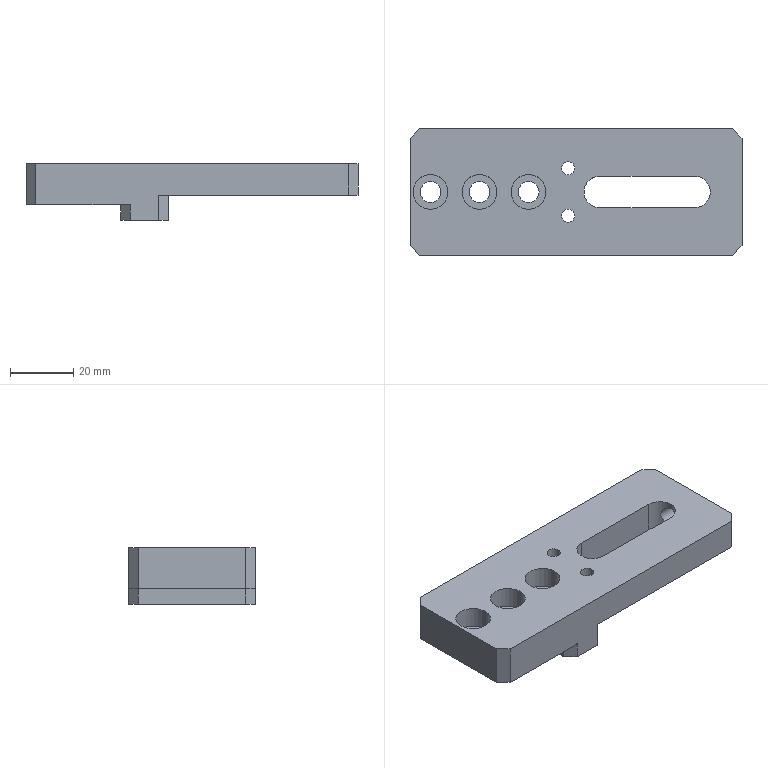Part | SolidWorks | features HoleWzd 3, ICE 3, Chamfer 1, Cut 1, Extrusion 1 | 1 solid | 47 faces | box 105 x 40 x 18 mm | volume 42827 mm3 | plane 24 | cylinder 23 | commonest cylinder face diameters 6.6 x8 11 x6 10 x5 4.2 x4
STEP:
#1=CARTESIAN_POINT('',(-0.4,7.5,8.));
#2=VERTEX_POINT('',#1);
#3=CARTESIAN_POINT('',(-4.6,7.5,8.));
#4=VERTEX_POINT('',#3);
#5=CARTESIAN_POINT('',(-2.5,7.5,8.));
#6=DIRECTION('',(0.,0.,-1.));
#7=DIRECTION('',(-1.,0.,0.));
#8=AXIS2_PLACEMENT_3D('',#5,#6,#7);
#9=CIRCLE('',#8,2.1);
#10=EDGE_CURVE('',#2,#4,#9,.T.);
#11=ORIENTED_EDGE('',*,*,#10,.T.);
#12=CARTESIAN_POINT('',(-4.6,7.5,18.));
#13=VERTEX_POINT('',#12);
#14=CARTESIAN_POINT('',(-4.6,7.5,18.));
#15=DIRECTION('',(0.,0.,1.));
#16=VECTOR('',#15,1000.);
#17=LINE('',#14,#16);
#18=EDGE_CURVE('',#4,#13,#17,.T.);
#19=ORIENTED_EDGE('',*,*,#18,.T.);
#20=CARTESIAN_POINT('',(-0.4,7.5,18.));
#21=VERTEX_POINT('',#20);
#22=CARTESIAN_POINT('',(-2.5,7.5,18.));
#23=DIRECTION('',(0.,0.,1.));
#24=DIRECTION('',(1.,0.,0.));
#25=AXIS2_PLACEMENT_3D('',#22,#23,#24);
#26=CIRCLE('',#25,2.1);
#27=EDGE_CURVE('',#13,#21,#26,.T.);
#28=ORIENTED_EDGE('',*,*,#27,.T.);
#29=CARTESIAN_POINT('',(-0.4,7.5,18.));
#30=DIRECTION('',(0.,0.,1.));
#31=VECTOR('',#30,1000.);
#32=LINE('',#29,#31);
#33=EDGE_CURVE('',#2,#21,#32,.T.);
#34=ORIENTED_EDGE('',*,*,#33,.F.);
#35=EDGE_LOOP('',(#11,#19,#28,#34));
#36=FACE_OUTER_BOUND('',#35,.T.);
#37=CARTESIAN_POINT('',(-2.5,7.5,18.));
#38=DIRECTION('',(0.,0.,1.));
#39=DIRECTION('',(1.,0.,0.));
#40=AXIS2_PLACEMENT_3D('',#37,#38,#39);
#41=CYLINDRICAL_SURFACE('',#40,2.1);
#42=ADVANCED_FACE('',(#36),#41,.F.);
#43=CARTESIAN_POINT('',(-0.4,-7.5,8.));
#44=VERTEX_POINT('',#43);
#45=CARTESIAN_POINT('',(-4.6,-7.5,8.));
#46=VERTEX_POINT('',#45);
#47=CARTESIAN_POINT('',(-2.5,-7.5,8.));
#48=DIRECTION('',(0.,0.,-1.));
#49=DIRECTION('',(-1.,0.,0.));
#50=AXIS2_PLACEMENT_3D('',#47,#48,#49);
#51=CIRCLE('',#50,2.1);
#52=EDGE_CURVE('',#44,#46,#51,.T.);
#53=ORIENTED_EDGE('',*,*,#52,.T.);
#54=CARTESIAN_POINT('',(-4.6,-7.5,18.));
#55=VERTEX_POINT('',#54);
#56=CARTESIAN_POINT('',(-4.6,-7.5,18.));
#57=DIRECTION('',(0.,0.,1.));
#58=VECTOR('',#57,1000.);
#59=LINE('',#56,#58);
#60=EDGE_CURVE('',#46,#55,#59,.T.);
#61=ORIENTED_EDGE('',*,*,#60,.T.);
#62=CARTESIAN_POINT('',(-0.4,-7.5,18.));
#63=VERTEX_POINT('',#62);
#64=CARTESIAN_POINT('',(-2.5,-7.5,18.));
#65=DIRECTION('',(0.,0.,1.));
#66=DIRECTION('',(1.,0.,0.));
#67=AXIS2_PLACEMENT_3D('',#64,#65,#66);
#68=CIRCLE('',#67,2.1);
#69=EDGE_CURVE('',#55,#63,#68,.T.);
#70=ORIENTED_EDGE('',*,*,#69,.T.);
#71=CARTESIAN_POINT('',(-0.4,-7.5,18.));
#72=DIRECTION('',(0.,0.,1.));
#73=VECTOR('',#72,1000.);
#74=LINE('',#71,#73);
#75=EDGE_CURVE('',#44,#63,#74,.T.);
#76=ORIENTED_EDGE('',*,*,#75,.F.);
#77=EDGE_LOOP('',(#53,#61,#70,#76));
#78=FACE_OUTER_BOUND('',#77,.T.);
#79=CARTESIAN_POINT('',(-2.5,-7.5,18.));
#80=DIRECTION('',(0.,0.,1.));
#81=DIRECTION('',(1.,0.,0.));
#82=AXIS2_PLACEMENT_3D('',#79,#80,#81);
#83=CYLINDRICAL_SURFACE('',#82,2.1);
#84=ADVANCED_FACE('',(#78),#83,.F.);
#85=CARTESIAN_POINT('',(42.5,0.,16.3));
#86=VERTEX_POINT('',#85);
#87=CARTESIAN_POINT('',(42.5,0.,9.7));
#88=VERTEX_POINT('',#87);
#89=CARTESIAN_POINT('',(42.5,0.,16.3));
#90=CARTESIAN_POINT('',(42.5,-0.222,16.3));
#91=CARTESIAN_POINT('',(42.485,-0.447,16.277));
#92=CARTESIAN_POINT('',(42.427,-0.8816,16.188));
#93=CARTESIAN_POINT('',(42.384,-1.09,16.122));
#94=CARTESIAN_POINT('',(42.277,-1.492,15.952));
#95=CARTESIAN_POINT('',(42.213,-1.681,15.848));
#96=CARTESIAN_POINT('',(42.073,-2.031,15.61));
#97=CARTESIAN_POINT('',(41.996,-2.195,15.473));
#98=CARTESIAN_POINT('',(41.84,-2.489,15.177));
#99=CARTESIAN_POINT('',(41.76,-2.621,15.016));
#100=CARTESIAN_POINT('',(41.607,-2.856,14.667));
#101=CARTESIAN_POINT('',(41.533,-2.958,14.479));
#102=CARTESIAN_POINT('',(41.406,-3.123,14.086));
#103=CARTESIAN_POINT('',(41.352,-3.189,13.878));
#104=CARTESIAN_POINT('',(41.276,-3.277,13.444));
#105=CARTESIAN_POINT('',(41.256,-3.3,13.223));
#106=CARTESIAN_POINT('',(41.256,-3.3,12.774));
#107=CARTESIAN_POINT('',(41.277,-3.277,12.55));
#108=CARTESIAN_POINT('',(41.352,-3.188,12.119));
#109=CARTESIAN_POINT('',(41.407,-3.122,11.909));
#110=CARTESIAN_POINT('',(41.598,-2.872,11.32));
#111=CARTESIAN_POINT('',(41.764,-2.633,10.967));
#112=CARTESIAN_POINT('',(41.997,-2.191,10.524));
#113=CARTESIAN_POINT('',(42.074,-2.028,10.388));
#114=CARTESIAN_POINT('',(42.214,-1.677,10.15));
#115=CARTESIAN_POINT('',(42.277,-1.49,10.048));
#116=CARTESIAN_POINT('',(42.383,-1.094,9.879));
#117=CARTESIAN_POINT('',(42.427,-0.8814,9.812));
#118=CARTESIAN_POINT('',(42.485,-0.4473,9.723));
#119=CARTESIAN_POINT('',(42.5,-0.2253,9.7));
#120=CARTESIAN_POINT('',(42.5,0.,9.7));
#121=B_SPLINE_CURVE_WITH_KNOTS('',3,(#89,#90,#91,#92,#93,#94,#95,#96,#97,#98,#99,#100,#101,#102,#103,#104,#105,#106,#107,#108,#109,#110,#111,#112,#113,#114,#115,#116,#117,#118,#119,#120),.UNSPECIFIED.,.F.,.F.,(4,2,2,2,2,2,2,2,2,2,2,2,2,2,2,4),(0.01066,0.01132,0.01199,0.01265,0.01332,0.01398,0.01465,0.01531,0.01598,0.01664,0.01731,0.01864,0.0193,0.01997,0.02063,0.0213),.UNSPECIFIED.);
#122=EDGE_CURVE('',#86,#88,#121,.T.);
#123=ORIENTED_EDGE('',*,*,#122,.F.);
#124=CARTESIAN_POINT('',(52.5,0.,16.3));
#125=VERTEX_POINT('',#124);
#126=CARTESIAN_POINT('',(52.5,0.,16.3));
#127=DIRECTION('',(1.,0.,0.));
#128=VECTOR('',#127,1000.);
#129=LINE('',#126,#128);
#130=EDGE_CURVE('',#86,#125,#129,.T.);
#131=ORIENTED_EDGE('',*,*,#130,.T.);
#132=CARTESIAN_POINT('',(52.5,0.,9.7));
#133=VERTEX_POINT('',#132);
#134=CARTESIAN_POINT('',(52.5,0.,13.));
#135=DIRECTION('',(1.,0.,0.));
#136=DIRECTION('',(0.,0.,-1.));
#137=AXIS2_PLACEMENT_3D('',#134,#135,#136);
#138=CIRCLE('',#137,3.3);
#139=EDGE_CURVE('',#125,#133,#138,.T.);
#140=ORIENTED_EDGE('',*,*,#139,.T.);
#141=CARTESIAN_POINT('',(52.5,0.,9.7));
#142=DIRECTION('',(1.,0.,0.));
#143=VECTOR('',#142,1000.);
#144=LINE('',#141,#143);
#145=EDGE_CURVE('',#88,#133,#144,.T.);
#146=ORIENTED_EDGE('',*,*,#145,.F.);
#147=EDGE_LOOP('',(#123,#131,#140,#146));
#148=FACE_OUTER_BOUND('',#147,.T.);
#149=CARTESIAN_POINT('',(52.5,0.,13.));
#150=DIRECTION('',(1.,0.,0.));
#151=DIRECTION('',(0.,0.,-1.));
#152=AXIS2_PLACEMENT_3D('',#149,#150,#151);
#153=CYLINDRICAL_SURFACE('',#152,3.3);
#154=ADVANCED_FACE('',(#148),#153,.F.);
#155=CARTESIAN_POINT('',(37.5,5.,8.));
#156=VERTEX_POINT('',#155);
#157=CARTESIAN_POINT('',(42.5,0.,8.));
#158=VERTEX_POINT('',#157);
#159=CARTESIAN_POINT('',(37.5,0.,8.));
#160=DIRECTION('',(0.,0.,-1.));
#161=DIRECTION('',(-1.,0.,0.));
#162=AXIS2_PLACEMENT_3D('',#159,#160,#161);
#163=CIRCLE('',#162,5.);
#164=EDGE_CURVE('',#156,#158,#163,.T.);
#165=ORIENTED_EDGE('',*,*,#164,.T.);
#166=CARTESIAN_POINT('',(42.5,0.,0.));
#167=DIRECTION('',(0.,0.,1.));
#168=VECTOR('',#167,1000.);
#169=LINE('',#166,#168);
#170=EDGE_CURVE('',#158,#88,#169,.T.);
#171=ORIENTED_EDGE('',*,*,#170,.T.);
#172=CARTESIAN_POINT('',(42.5,0.,9.7));
#173=CARTESIAN_POINT('',(42.5,0.2256,9.7));
#174=CARTESIAN_POINT('',(42.485,0.4462,9.723));
#175=CARTESIAN_POINT('',(42.427,0.8783,9.811));
#176=CARTESIAN_POINT('',(42.384,1.091,9.878));
#177=CARTESIAN_POINT('',(42.224,1.689,10.132));
#178=CARTESIAN_POINT('',(42.075,2.045,10.376));
#179=CARTESIAN_POINT('',(41.841,2.487,10.82));
#180=CARTESIAN_POINT('',(41.76,2.621,10.984));
#181=CARTESIAN_POINT('',(41.608,2.854,11.331));
#182=CARTESIAN_POINT('',(41.535,2.955,11.515));
#183=CARTESIAN_POINT('',(41.408,3.121,11.908));
#184=CARTESIAN_POINT('',(41.353,3.188,12.118));
#185=CARTESIAN_POINT('',(41.296,3.254,12.441));
#186=CARTESIAN_POINT('',(41.282,3.271,12.55));
#187=CARTESIAN_POINT('',(41.262,3.294,12.772));
#188=CARTESIAN_POINT('',(41.256,3.3,12.885));
#189=CARTESIAN_POINT('',(41.256,3.3,13.221));
#190=CARTESIAN_POINT('',(41.276,3.278,13.441));
#191=CARTESIAN_POINT('',(41.351,3.189,13.876));
#192=CARTESIAN_POINT('',(41.405,3.124,14.084));
#193=CARTESIAN_POINT('',(41.533,2.957,14.48));
#194=CARTESIAN_POINT('',(41.607,2.855,14.668));
#195=CARTESIAN_POINT('',(41.76,2.621,15.016));
#196=CARTESIAN_POINT('',(41.84,2.488,15.178));
#197=CARTESIAN_POINT('',(41.997,2.191,15.476));
#198=CARTESIAN_POINT('',(42.073,2.03,15.61));
#199=CARTESIAN_POINT('',(42.212,1.682,15.847));
#200=CARTESIAN_POINT('',(42.277,1.491,15.952));
#201=CARTESIAN_POINT('',(42.384,1.091,16.122));
#202=CARTESIAN_POINT('',(42.426,0.8826,16.188));
#203=CARTESIAN_POINT('',(42.485,0.4472,16.277));
#204=CARTESIAN_POINT('',(42.5,0.2223,16.3));
#205=CARTESIAN_POINT('',(42.5,0.,16.3));
#206=B_SPLINE_CURVE_WITH_KNOTS('',3,(#172,#173,#174,#175,#176,#177,#178,#179,#180,#181,#182,#183,#184,#185,#186,#187,#188,#189,#190,#191,#192,#193,#194,#195,#196,#197,#198,#199,#200,#201,#202,#203,#204,#205),.UNSPECIFIED.,.F.,.F.,(4,2,2,2,2,2,2,2,2,2,2,2,2,2,2,2,4),(0.,0.000666,0.001332,0.002664,0.00333,0.003996,0.004662,0.004995,0.005328,0.005994,0.00666,0.007326,0.007992,0.008658,0.009324,0.00999,0.01066),.UNSPECIFIED.);
#207=EDGE_CURVE('',#88,#86,#206,.T.);
#208=ORIENTED_EDGE('',*,*,#207,.T.);
#209=CARTESIAN_POINT('',(42.5,0.,18.));
#210=VERTEX_POINT('',#209);
#211=CARTESIAN_POINT('',(42.5,0.,0.));
#212=DIRECTION('',(0.,0.,1.));
#213=VECTOR('',#212,1000.);
#214=LINE('',#211,#213);
#215=EDGE_CURVE('',#86,#210,#214,.T.);
#216=ORIENTED_EDGE('',*,*,#215,.T.);
#217=CARTESIAN_POINT('',(37.5,5.,18.));
#218=VERTEX_POINT('',#217);
#219=CARTESIAN_POINT('',(37.5,0.,18.));
#220=DIRECTION('',(0.,0.,1.));
#221=DIRECTION('',(1.,0.,0.));
#222=AXIS2_PLACEMENT_3D('',#219,#220,#221);
#223=CIRCLE('',#222,5.);
#224=EDGE_CURVE('',#210,#218,#223,.T.);
#225=ORIENTED_EDGE('',*,*,#224,.T.);
#226=CARTESIAN_POINT('',(37.5,5.,0.));
#227=DIRECTION('',(0.,0.,1.));
#228=VECTOR('',#227,1000.);
#229=LINE('',#226,#228);
#230=EDGE_CURVE('',#156,#218,#229,.T.);
#231=ORIENTED_EDGE('',*,*,#230,.F.);
#232=EDGE_LOOP('',(#165,#171,#208,#216,#225,#231));
#233=FACE_OUTER_BOUND('',#232,.T.);
#234=CARTESIAN_POINT('',(37.5,0.,0.));
#235=DIRECTION('',(0.,0.,1.));
#236=DIRECTION('',(1.,0.,0.));
#237=AXIS2_PLACEMENT_3D('',#234,#235,#236);
#238=CYLINDRICAL_SURFACE('',#237,5.);
#239=ADVANCED_FACE('',(#233),#238,.F.);
#240=CARTESIAN_POINT('',(-10.,0.,2.));
#241=VERTEX_POINT('',#240);
#242=CARTESIAN_POINT('',(-20.,0.,2.));
#243=VERTEX_POINT('',#242);
#244=CARTESIAN_POINT('',(-15.,0.,2.));
#245=DIRECTION('',(0.,0.,-1.));
#246=DIRECTION('',(-1.,0.,0.));
#247=AXIS2_PLACEMENT_3D('',#244,#245,#246);
#248=CIRCLE('',#247,5.);
#249=EDGE_CURVE('',#241,#243,#248,.T.);
#250=ORIENTED_EDGE('',*,*,#249,.F.);
#251=CARTESIAN_POINT('',(-10.,0.,0.));
#252=VERTEX_POINT('',#251);
#253=CARTESIAN_POINT('',(-10.,0.,2.));
#254=DIRECTION('',(0.,0.,-1.));
#255=VECTOR('',#254,1000.);
#256=LINE('',#253,#255);
#257=EDGE_CURVE('',#241,#252,#256,.T.);
#258=ORIENTED_EDGE('',*,*,#257,.T.);
#259=CARTESIAN_POINT('',(-20.,0.,0.));
#260=VERTEX_POINT('',#259);
#261=CARTESIAN_POINT('',(-15.,0.,0.));
#262=DIRECTION('',(0.,0.,-1.));
#263=DIRECTION('',(-1.,0.,0.));
#264=AXIS2_PLACEMENT_3D('',#261,#262,#263);
#265=CIRCLE('',#264,5.);
#266=EDGE_CURVE('',#252,#260,#265,.T.);
#267=ORIENTED_EDGE('',*,*,#266,.T.);
#268=CARTESIAN_POINT('',(-20.,0.,2.));
#269=DIRECTION('',(0.,0.,-1.));
#270=VECTOR('',#269,1000.);
#271=LINE('',#268,#270);
#272=EDGE_CURVE('',#243,#260,#271,.T.);
#273=ORIENTED_EDGE('',*,*,#272,.F.);
#274=EDGE_LOOP('',(#250,#258,#267,#273));
#275=FACE_OUTER_BOUND('',#274,.T.);
#276=CARTESIAN_POINT('',(-15.,0.,2.));
#277=DIRECTION('',(0.,0.,-1.));
#278=DIRECTION('',(-1.,0.,0.));
#279=AXIS2_PLACEMENT_3D('',#276,#277,#278);
#280=CYLINDRICAL_SURFACE('',#279,5.);
#281=ADVANCED_FACE('',(#275),#280,.F.);
#282=CARTESIAN_POINT('',(-51.5,0.,11.2));
#283=VERTEX_POINT('',#282);
#284=CARTESIAN_POINT('',(-40.5,0.,11.2));
#285=VERTEX_POINT('',#284);
#286=CARTESIAN_POINT('',(-46.,0.,11.2));
#287=DIRECTION('',(0.,0.,1.));
#288=DIRECTION('',(1.,0.,0.));
#289=AXIS2_PLACEMENT_3D('',#286,#287,#288);
#290=CIRCLE('',#289,5.5);
#291=EDGE_CURVE('',#283,#285,#290,.T.);
#292=ORIENTED_EDGE('',*,*,#291,.F.);
#293=CARTESIAN_POINT('',(-51.5,0.,18.));
#294=VERTEX_POINT('',#293);
#295=CARTESIAN_POINT('',(-51.5,0.,18.));
#296=DIRECTION('',(0.,0.,1.));
#297=VECTOR('',#296,1000.);
#298=LINE('',#295,#297);
#299=EDGE_CURVE('',#283,#294,#298,.T.);
#300=ORIENTED_EDGE('',*,*,#299,.T.);
#301=CARTESIAN_POINT('',(-40.5,0.,18.));
#302=VERTEX_POINT('',#301);
#303=CARTESIAN_POINT('',(-46.,0.,18.));
#304=DIRECTION('',(0.,0.,1.));
#305=DIRECTION('',(1.,0.,0.));
#306=AXIS2_PLACEMENT_3D('',#303,#304,#305);
#307=CIRCLE('',#306,5.5);
#308=EDGE_CURVE('',#294,#302,#307,.T.);
#309=ORIENTED_EDGE('',*,*,#308,.T.);
#310=CARTESIAN_POINT('',(-40.5,0.,18.));
#311=DIRECTION('',(0.,0.,1.));
#312=VECTOR('',#311,1000.);
#313=LINE('',#310,#312);
#314=EDGE_CURVE('',#285,#302,#313,.T.);
#315=ORIENTED_EDGE('',*,*,#314,.F.);
#316=EDGE_LOOP('',(#292,#300,#309,#315));
#317=FACE_OUTER_BOUND('',#316,.T.);
#318=CARTESIAN_POINT('',(-46.,0.,18.));
#319=DIRECTION('',(0.,0.,1.));
#320=DIRECTION('',(1.,0.,0.));
#321=AXIS2_PLACEMENT_3D('',#318,#319,#320);
#322=CYLINDRICAL_SURFACE('',#321,5.5);
#323=ADVANCED_FACE('',(#317),#322,.F.);
#324=CARTESIAN_POINT('',(-49.3,0.,5.));
#325=VERTEX_POINT('',#324);
#326=CARTESIAN_POINT('',(-42.7,0.,5.));
#327=VERTEX_POINT('',#326);
#328=CARTESIAN_POINT('',(-46.,0.,5.));
#329=DIRECTION('',(0.,0.,1.));
#330=DIRECTION('',(1.,0.,0.));
#331=AXIS2_PLACEMENT_3D('',#328,#329,#330);
#332=CIRCLE('',#331,3.3);
#333=EDGE_CURVE('',#325,#327,#332,.T.);
#334=ORIENTED_EDGE('',*,*,#333,.F.);
#335=CARTESIAN_POINT('',(-49.3,0.,11.2));
#336=VERTEX_POINT('',#335);
#337=CARTESIAN_POINT('',(-49.3,0.,18.));
#338=DIRECTION('',(0.,0.,1.));
#339=VECTOR('',#338,1000.);
#340=LINE('',#337,#339);
#341=EDGE_CURVE('',#325,#336,#340,.T.);
#342=ORIENTED_EDGE('',*,*,#341,.T.);
#343=CARTESIAN_POINT('',(-42.7,0.,11.2));
#344=VERTEX_POINT('',#343);
#345=CARTESIAN_POINT('',(-46.,0.,11.2));
#346=DIRECTION('',(0.,0.,1.));
#347=DIRECTION('',(1.,0.,0.));
#348=AXIS2_PLACEMENT_3D('',#345,#346,#347);
#349=CIRCLE('',#348,3.3);
#350=EDGE_CURVE('',#336,#344,#349,.T.);
#351=ORIENTED_EDGE('',*,*,#350,.T.);
#352=CARTESIAN_POINT('',(-42.7,0.,18.));
#353=DIRECTION('',(0.,0.,1.));
#354=VECTOR('',#353,1000.);
#355=LINE('',#352,#354);
#356=EDGE_CURVE('',#327,#344,#355,.T.);
#357=ORIENTED_EDGE('',*,*,#356,.F.);
#358=EDGE_LOOP('',(#334,#342,#351,#357));
#359=FACE_OUTER_BOUND('',#358,.T.);
#360=CARTESIAN_POINT('',(-46.,0.,18.));
#361=DIRECTION('',(0.,0.,1.));
#362=DIRECTION('',(1.,0.,0.));
#363=AXIS2_PLACEMENT_3D('',#360,#361,#362);
#364=CYLINDRICAL_SURFACE('',#363,3.3);
#365=ADVANCED_FACE('',(#359),#364,.F.);
#366=CARTESIAN_POINT('',(-36.,0.,11.2));
#367=VERTEX_POINT('',#366);
#368=CARTESIAN_POINT('',(-25.,0.,11.2));
#369=VERTEX_POINT('',#368);
#370=CARTESIAN_POINT('',(-30.5,0.,11.2));
#371=DIRECTION('',(0.,0.,1.));
#372=DIRECTION('',(1.,0.,0.));
#373=AXIS2_PLACEMENT_3D('',#370,#371,#372);
#374=CIRCLE('',#373,5.5);
#375=EDGE_CURVE('',#367,#369,#374,.T.);
#376=ORIENTED_EDGE('',*,*,#375,.F.);
#377=CARTESIAN_POINT('',(-36.,0.,18.));
#378=VERTEX_POINT('',#377);
#379=CARTESIAN_POINT('',(-36.,0.,18.));
#380=DIRECTION('',(0.,0.,1.));
#381=VECTOR('',#380,1000.);
#382=LINE('',#379,#381);
#383=EDGE_CURVE('',#367,#378,#382,.T.);
#384=ORIENTED_EDGE('',*,*,#383,.T.);
#385=CARTESIAN_POINT('',(-25.,0.,18.));
#386=VERTEX_POINT('',#385);
#387=CARTESIAN_POINT('',(-30.5,0.,18.));
#388=DIRECTION('',(0.,0.,1.));
#389=DIRECTION('',(1.,0.,0.));
#390=AXIS2_PLACEMENT_3D('',#387,#388,#389);
#391=CIRCLE('',#390,5.5);
#392=EDGE_CURVE('',#378,#386,#391,.T.);
#393=ORIENTED_EDGE('',*,*,#392,.T.);
#394=CARTESIAN_POINT('',(-25.,0.,18.));
#395=DIRECTION('',(0.,0.,1.));
#396=VECTOR('',#395,1000.);
#397=LINE('',#394,#396);
#398=EDGE_CURVE('',#369,#386,#397,.T.);
#399=ORIENTED_EDGE('',*,*,#398,.F.);
#400=EDGE_LOOP('',(#376,#384,#393,#399));
#401=FACE_OUTER_BOUND('',#400,.T.);
#402=CARTESIAN_POINT('',(-30.5,0.,18.));
#403=DIRECTION('',(0.,0.,1.));
#404=DIRECTION('',(1.,0.,0.));
#405=AXIS2_PLACEMENT_3D('',#402,#403,#404);
#406=CYLINDRICAL_SURFACE('',#405,5.5);
#407=ADVANCED_FACE('',(#401),#406,.F.);
#408=CARTESIAN_POINT('',(-33.8,0.,5.));
#409=VERTEX_POINT('',#408);
#410=CARTESIAN_POINT('',(-27.2,0.,5.));
#411=VERTEX_POINT('',#410);
#412=CARTESIAN_POINT('',(-30.5,0.,5.));
#413=DIRECTION('',(0.,0.,1.));
#414=DIRECTION('',(1.,0.,0.));
#415=AXIS2_PLACEMENT_3D('',#412,#413,#414);
#416=CIRCLE('',#415,3.3);
#417=EDGE_CURVE('',#409,#411,#416,.T.);
#418=ORIENTED_EDGE('',*,*,#417,.F.);
#419=CARTESIAN_POINT('',(-33.8,0.,11.2));
#420=VERTEX_POINT('',#419);
#421=CARTESIAN_POINT('',(-33.8,0.,18.));
#422=DIRECTION('',(0.,0.,1.));
#423=VECTOR('',#422,1000.);
#424=LINE('',#421,#423);
#425=EDGE_CURVE('',#409,#420,#424,.T.);
#426=ORIENTED_EDGE('',*,*,#425,.T.);
#427=CARTESIAN_POINT('',(-27.2,0.,11.2));
#428=VERTEX_POINT('',#427);
#429=CARTESIAN_POINT('',(-30.5,0.,11.2));
#430=DIRECTION('',(0.,0.,1.));
#431=DIRECTION('',(1.,0.,0.));
#432=AXIS2_PLACEMENT_3D('',#429,#430,#431);
#433=CIRCLE('',#432,3.3);
#434=EDGE_CURVE('',#420,#428,#433,.T.);
#435=ORIENTED_EDGE('',*,*,#434,.T.);
#436=CARTESIAN_POINT('',(-27.2,0.,18.));
#437=DIRECTION('',(0.,0.,1.));
#438=VECTOR('',#437,1000.);
#439=LINE('',#436,#438);
#440=EDGE_CURVE('',#411,#428,#439,.T.);
#441=ORIENTED_EDGE('',*,*,#440,.F.);
#442=EDGE_LOOP('',(#418,#426,#435,#441));
#443=FACE_OUTER_BOUND('',#442,.T.);
#444=CARTESIAN_POINT('',(-30.5,0.,18.));
#445=DIRECTION('',(0.,0.,1.));
#446=DIRECTION('',(1.,0.,0.));
#447=AXIS2_PLACEMENT_3D('',#444,#445,#446);
#448=CYLINDRICAL_SURFACE('',#447,3.3);
#449=ADVANCED_FACE('',(#443),#448,.F.);
#450=CARTESIAN_POINT('',(-20.5,0.,11.2));
#451=VERTEX_POINT('',#450);
#452=CARTESIAN_POINT('',(-9.5,0.,11.2));
#453=VERTEX_POINT('',#452);
#454=CARTESIAN_POINT('',(-15.,0.,11.2));
#455=DIRECTION('',(0.,0.,1.));
#456=DIRECTION('',(1.,0.,0.));
#457=AXIS2_PLACEMENT_3D('',#454,#455,#456);
#458=CIRCLE('',#457,5.5);
#459=EDGE_CURVE('',#451,#453,#458,.T.);
#460=ORIENTED_EDGE('',*,*,#459,.F.);
#461=CARTESIAN_POINT('',(-20.5,0.,18.));
#462=VERTEX_POINT('',#461);
#463=CARTESIAN_POINT('',(-20.5,0.,18.));
#464=DIRECTION('',(0.,0.,1.));
#465=VECTOR('',#464,1000.);
#466=LINE('',#463,#465);
#467=EDGE_CURVE('',#451,#462,#466,.T.);
#468=ORIENTED_EDGE('',*,*,#467,.T.);
#469=CARTESIAN_POINT('',(-9.5,0.,18.));
#470=VERTEX_POINT('',#469);
#471=CARTESIAN_POINT('',(-15.,0.,18.));
#472=DIRECTION('',(0.,0.,1.));
#473=DIRECTION('',(1.,0.,0.));
#474=AXIS2_PLACEMENT_3D('',#471,#472,#473);
#475=CIRCLE('',#474,5.5);
#476=EDGE_CURVE('',#462,#470,#475,.T.);
#477=ORIENTED_EDGE('',*,*,#476,.T.);
#478=CARTESIAN_POINT('',(-9.5,0.,18.));
#479=DIRECTION('',(0.,0.,1.));
#480=VECTOR('',#479,1000.);
#481=LINE('',#478,#480);
#482=EDGE_CURVE('',#453,#470,#481,.T.);
#483=ORIENTED_EDGE('',*,*,#482,.F.);
#484=EDGE_LOOP('',(#460,#468,#477,#483));
#485=FACE_OUTER_BOUND('',#484,.T.);
#486=CARTESIAN_POINT('',(-15.,0.,18.));
#487=DIRECTION('',(0.,0.,1.));
#488=DIRECTION('',(1.,0.,0.));
#489=AXIS2_PLACEMENT_3D('',#486,#487,#488);
#490=CYLINDRICAL_SURFACE('',#489,5.5);
#491=ADVANCED_FACE('',(#485),#490,.F.);
#492=CARTESIAN_POINT('',(-18.3,0.,2.));
#493=VERTEX_POINT('',#492);
#494=CARTESIAN_POINT('',(-11.7,0.,2.));
#495=VERTEX_POINT('',#494);
#496=CARTESIAN_POINT('',(-15.,0.,2.));
#497=DIRECTION('',(0.,0.,1.));
#498=DIRECTION('',(-1.,0.,0.));
#499=AXIS2_PLACEMENT_3D('',#496,#497,#498);
#500=CIRCLE('',#499,3.3);
#501=EDGE_CURVE('',#493,#495,#500,.T.);
#502=ORIENTED_EDGE('',*,*,#501,.F.);
#503=CARTESIAN_POINT('',(-18.3,0.,11.2));
#504=VERTEX_POINT('',#503);
#505=CARTESIAN_POINT('',(-18.3,0.,18.));
#506=DIRECTION('',(0.,0.,1.));
#507=VECTOR('',#506,1000.);
#508=LINE('',#505,#507);
#509=EDGE_CURVE('',#493,#504,#508,.T.);
#510=ORIENTED_EDGE('',*,*,#509,.T.);
#511=CARTESIAN_POINT('',(-11.7,0.,11.2));
#512=VERTEX_POINT('',#511);
#513=CARTESIAN_POINT('',(-15.,0.,11.2));
#514=DIRECTION('',(0.,0.,1.));
#515=DIRECTION('',(1.,0.,0.));
#516=AXIS2_PLACEMENT_3D('',#513,#514,#515);
#517=CIRCLE('',#516,3.3);
#518=EDGE_CURVE('',#504,#512,#517,.T.);
#519=ORIENTED_EDGE('',*,*,#518,.T.);
#520=CARTESIAN_POINT('',(-11.7,0.,18.));
#521=DIRECTION('',(0.,0.,1.));
#522=VECTOR('',#521,1000.);
#523=LINE('',#520,#522);
#524=EDGE_CURVE('',#495,#512,#523,.T.);
#525=ORIENTED_EDGE('',*,*,#524,.F.);
#526=EDGE_LOOP('',(#502,#510,#519,#525));
#527=FACE_OUTER_BOUND('',#526,.T.);
#528=CARTESIAN_POINT('',(-15.,0.,18.));
#529=DIRECTION('',(0.,0.,1.));
#530=DIRECTION('',(1.,0.,0.));
#531=AXIS2_PLACEMENT_3D('',#528,#529,#530);
#532=CYLINDRICAL_SURFACE('',#531,3.3);
#533=ADVANCED_FACE('',(#527),#532,.F.);
#534=ORIENTED_EDGE('',*,*,#509,.F.);
#535=CARTESIAN_POINT('',(-15.,0.,2.));
#536=DIRECTION('',(0.,0.,1.));
#537=DIRECTION('',(-1.,0.,0.));
#538=AXIS2_PLACEMENT_3D('',#535,#536,#537);
#539=CIRCLE('',#538,3.3);
#540=EDGE_CURVE('',#495,#493,#539,.T.);
#541=ORIENTED_EDGE('',*,*,#540,.F.);
#542=ORIENTED_EDGE('',*,*,#524,.T.);
#543=CARTESIAN_POINT('',(-15.,0.,11.2));
#544=DIRECTION('',(0.,0.,1.));
#545=DIRECTION('',(1.,0.,0.));
#546=AXIS2_PLACEMENT_3D('',#543,#544,#545);
#547=CIRCLE('',#546,3.3);
#548=EDGE_CURVE('',#512,#504,#547,.T.);
#549=ORIENTED_EDGE('',*,*,#548,.T.);
#550=EDGE_LOOP('',(#534,#541,#542,#549));
#551=FACE_OUTER_BOUND('',#550,.T.);
#552=CARTESIAN_POINT('',(-15.,0.,18.));
#553=DIRECTION('',(0.,0.,1.));
#554=DIRECTION('',(1.,0.,0.));
#555=AXIS2_PLACEMENT_3D('',#552,#553,#554);
#556=CYLINDRICAL_SURFACE('',#555,3.3);
#557=ADVANCED_FACE('',(#551),#556,.F.);
#558=CARTESIAN_POINT('',(52.5,0.,13.));
#559=DIRECTION('',(1.,0.,0.));
#560=DIRECTION('',(0.,0.,-1.));
#561=AXIS2_PLACEMENT_3D('',#558,#559,#560);
#562=CIRCLE('',#561,3.3);
#563=EDGE_CURVE('',#133,#125,#562,.T.);
#564=ORIENTED_EDGE('',*,*,#563,.F.);
#565=ORIENTED_EDGE('',*,*,#139,.F.);
#566=EDGE_LOOP('',(#564,#565));
#567=FACE_BOUND('',#566,.T.);
#568=CARTESIAN_POINT('',(52.5,-17.,18.));
#569=VERTEX_POINT('',#568);
#570=CARTESIAN_POINT('',(52.5,17.,18.));
#571=VERTEX_POINT('',#570);
#572=CARTESIAN_POINT('',(52.5,-20.,18.));
#573=DIRECTION('',(0.,1.,0.));
#574=VECTOR('',#573,1000.);
#575=LINE('',#572,#574);
#576=EDGE_CURVE('',#569,#571,#575,.T.);
#577=ORIENTED_EDGE('',*,*,#576,.F.);
#578=CARTESIAN_POINT('',(52.5,-17.,8.));
#579=VERTEX_POINT('',#578);
#580=CARTESIAN_POINT('',(52.5,-17.,18.));
#581=DIRECTION('',(0.,0.,-1.));
#582=VECTOR('',#581,1000.);
#583=LINE('',#580,#582);
#584=EDGE_CURVE('',#569,#579,#583,.T.);
#585=ORIENTED_EDGE('',*,*,#584,.T.);
#586=CARTESIAN_POINT('',(52.5,17.,8.));
#587=VERTEX_POINT('',#586);
#588=CARTESIAN_POINT('',(52.5,20.,8.));
#589=DIRECTION('',(0.,-1.,0.));
#590=VECTOR('',#589,1000.);
#591=LINE('',#588,#590);
#592=EDGE_CURVE('',#587,#579,#591,.T.);
#593=ORIENTED_EDGE('',*,*,#592,.F.);
#594=CARTESIAN_POINT('',(52.5,17.,18.));
#595=DIRECTION('',(0.,0.,1.));
#596=VECTOR('',#595,1000.);
#597=LINE('',#594,#596);
#598=EDGE_CURVE('',#587,#571,#597,.T.);
#599=ORIENTED_EDGE('',*,*,#598,.T.);
#600=EDGE_LOOP('',(#577,#585,#593,#599));
#601=FACE_OUTER_BOUND('',#600,.T.);
#602=CARTESIAN_POINT('',(52.5,-20.,18.));
#603=DIRECTION('',(-1.,0.,0.));
#604=DIRECTION('',(0.,0.,1.));
#605=AXIS2_PLACEMENT_3D('',#602,#603,#604);
#606=PLANE('',#605);
#607=ADVANCED_FACE('',(#567,#601),#606,.F.);
#608=CARTESIAN_POINT('',(-10.5,20.,8.));
#609=VERTEX_POINT('',#608);
#610=CARTESIAN_POINT('',(49.5,20.,8.));
#611=VERTEX_POINT('',#610);
#612=CARTESIAN_POINT('',(52.5,20.,8.));
#613=DIRECTION('',(1.,0.,0.));
#614=VECTOR('',#613,1000.);
#615=LINE('',#612,#614);
#616=EDGE_CURVE('',#609,#611,#615,.T.);
#617=ORIENTED_EDGE('',*,*,#616,.F.);
#618=CARTESIAN_POINT('',(-10.5,20.,0.));
#619=VERTEX_POINT('',#618);
#620=CARTESIAN_POINT('',(-10.5,20.,18.));
#621=DIRECTION('',(0.,0.,-1.));
#622=VECTOR('',#621,1000.);
#623=LINE('',#620,#622);
#624=EDGE_CURVE('',#609,#619,#623,.T.);
#625=ORIENTED_EDGE('',*,*,#624,.T.);
#626=CARTESIAN_POINT('',(-19.5,20.,0.));
#627=VERTEX_POINT('',#626);
#628=CARTESIAN_POINT('',(-52.5,20.,0.));
#629=DIRECTION('',(-1.,0.,0.));
#630=VECTOR('',#629,1000.);
#631=LINE('',#628,#630);
#632=EDGE_CURVE('',#619,#627,#631,.T.);
#633=ORIENTED_EDGE('',*,*,#632,.T.);
#634=CARTESIAN_POINT('',(-19.5,20.,5.));
#635=VERTEX_POINT('',#634);
#636=CARTESIAN_POINT('',(-19.5,20.,18.));
#637=DIRECTION('',(0.,0.,1.));
#638=VECTOR('',#637,1000.);
#639=LINE('',#636,#638);
#640=EDGE_CURVE('',#627,#635,#639,.T.);
#641=ORIENTED_EDGE('',*,*,#640,.T.);
#642=CARTESIAN_POINT('',(-49.5,20.,5.));
#643=VERTEX_POINT('',#642);
#644=CARTESIAN_POINT('',(-52.5,20.,5.));
#645=DIRECTION('',(1.,0.,0.));
#646=VECTOR('',#645,1000.);
#647=LINE('',#644,#646);
#648=EDGE_CURVE('',#643,#635,#647,.T.);
#649=ORIENTED_EDGE('',*,*,#648,.F.);
#650=CARTESIAN_POINT('',(-49.5,20.,18.));
#651=VERTEX_POINT('',#650);
#652=CARTESIAN_POINT('',(-49.5,20.,18.));
#653=DIRECTION('',(0.,0.,1.));
#654=VECTOR('',#653,1000.);
#655=LINE('',#652,#654);
#656=EDGE_CURVE('',#643,#651,#655,.T.);
#657=ORIENTED_EDGE('',*,*,#656,.T.);
#658=CARTESIAN_POINT('',(49.5,20.,18.));
#659=VERTEX_POINT('',#658);
#660=CARTESIAN_POINT('',(-52.5,20.,18.));
#661=DIRECTION('',(-1.,0.,0.));
#662=VECTOR('',#661,1000.);
#663=LINE('',#660,#662);
#664=EDGE_CURVE('',#659,#651,#663,.T.);
#665=ORIENTED_EDGE('',*,*,#664,.F.);
#666=CARTESIAN_POINT('',(49.5,20.,18.));
#667=DIRECTION('',(0.,0.,-1.));
#668=VECTOR('',#667,1000.);
#669=LINE('',#666,#668);
#670=EDGE_CURVE('',#659,#611,#669,.T.);
#671=ORIENTED_EDGE('',*,*,#670,.T.);
#672=EDGE_LOOP('',(#617,#625,#633,#641,#649,#657,#665,#671));
#673=FACE_OUTER_BOUND('',#672,.T.);
#674=CARTESIAN_POINT('',(-52.5,20.,18.));
#675=DIRECTION('',(0.,-1.,0.));
#676=DIRECTION('',(0.,0.,-1.));
#677=AXIS2_PLACEMENT_3D('',#674,#675,#676);
#678=PLANE('',#677);
#679=ADVANCED_FACE('',(#673),#678,.F.);
#680=CARTESIAN_POINT('',(-52.5,17.,18.));
#681=VERTEX_POINT('',#680);
#682=CARTESIAN_POINT('',(-52.5,-17.,18.));
#683=VERTEX_POINT('',#682);
#684=CARTESIAN_POINT('',(-52.5,-20.,18.));
#685=DIRECTION('',(0.,-1.,0.));
#686=VECTOR('',#685,1000.);
#687=LINE('',#684,#686);
#688=EDGE_CURVE('',#681,#683,#687,.T.);
#689=ORIENTED_EDGE('',*,*,#688,.F.);
#690=CARTESIAN_POINT('',(-52.5,17.,5.));
#691=VERTEX_POINT('',#690);
#692=CARTESIAN_POINT('',(-52.5,17.,18.));
#693=DIRECTION('',(0.,0.,-1.));
#694=VECTOR('',#693,1000.);
#695=LINE('',#692,#694);
#696=EDGE_CURVE('',#681,#691,#695,.T.);
#697=ORIENTED_EDGE('',*,*,#696,.T.);
#698=CARTESIAN_POINT('',(-52.5,-17.,5.));
#699=VERTEX_POINT('',#698);
#700=CARTESIAN_POINT('',(-52.5,20.,5.));
#701=DIRECTION('',(0.,1.,0.));
#702=VECTOR('',#701,1000.);
#703=LINE('',#700,#702);
#704=EDGE_CURVE('',#699,#691,#703,.T.);
#705=ORIENTED_EDGE('',*,*,#704,.F.);
#706=CARTESIAN_POINT('',(-52.5,-17.,18.));
#707=DIRECTION('',(0.,0.,1.));
#708=VECTOR('',#707,1000.);
#709=LINE('',#706,#708);
#710=EDGE_CURVE('',#699,#683,#709,.T.);
#711=ORIENTED_EDGE('',*,*,#710,.T.);
#712=EDGE_LOOP('',(#689,#697,#705,#711));
#713=FACE_OUTER_BOUND('',#712,.T.);
#714=CARTESIAN_POINT('',(-52.5,-20.,18.));
#715=DIRECTION('',(1.,0.,0.));
#716=DIRECTION('',(0.,0.,-1.));
#717=AXIS2_PLACEMENT_3D('',#714,#715,#716);
#718=PLANE('',#717);
#719=ADVANCED_FACE('',(#713),#718,.F.);
#720=CARTESIAN_POINT('',(-19.5,-20.,5.));
#721=VERTEX_POINT('',#720);
#722=CARTESIAN_POINT('',(-49.5,-20.,5.));
#723=VERTEX_POINT('',#722);
#724=CARTESIAN_POINT('',(-52.5,-20.,5.));
#725=DIRECTION('',(-1.,0.,0.));
#726=VECTOR('',#725,1000.);
#727=LINE('',#724,#726);
#728=EDGE_CURVE('',#721,#723,#727,.T.);
#729=ORIENTED_EDGE('',*,*,#728,.F.);
#730=CARTESIAN_POINT('',(-19.5,-20.,0.));
#731=VERTEX_POINT('',#730);
#732=CARTESIAN_POINT('',(-19.5,-20.,18.));
#733=DIRECTION('',(0.,0.,-1.));
#734=VECTOR('',#733,1000.);
#735=LINE('',#732,#734);
#736=EDGE_CURVE('',#721,#731,#735,.T.);
#737=ORIENTED_EDGE('',*,*,#736,.T.);
#738=CARTESIAN_POINT('',(-10.5,-20.,0.));
#739=VERTEX_POINT('',#738);
#740=CARTESIAN_POINT('',(-52.5,-20.,0.));
#741=DIRECTION('',(1.,0.,0.));
#742=VECTOR('',#741,1000.);
#743=LINE('',#740,#742);
#744=EDGE_CURVE('',#731,#739,#743,.T.);
#745=ORIENTED_EDGE('',*,*,#744,.T.);
#746=CARTESIAN_POINT('',(-10.5,-20.,8.));
#747=VERTEX_POINT('',#746);
#748=CARTESIAN_POINT('',(-10.5,-20.,18.));
#749=DIRECTION('',(0.,0.,1.));
#750=VECTOR('',#749,1000.);
#751=LINE('',#748,#750);
#752=EDGE_CURVE('',#739,#747,#751,.T.);
#753=ORIENTED_EDGE('',*,*,#752,.T.);
#754=CARTESIAN_POINT('',(49.5,-20.,8.));
#755=VERTEX_POINT('',#754);
#756=CARTESIAN_POINT('',(52.5,-20.,8.));
#757=DIRECTION('',(-1.,0.,0.));
#758=VECTOR('',#757,1000.);
#759=LINE('',#756,#758);
#760=EDGE_CURVE('',#755,#747,#759,.T.);
#761=ORIENTED_EDGE('',*,*,#760,.F.);
#762=CARTESIAN_POINT('',(49.5,-20.,18.));
#763=VERTEX_POINT('',#762);
#764=CARTESIAN_POINT('',(49.5,-20.,18.));
#765=DIRECTION('',(0.,0.,1.));
#766=VECTOR('',#765,1000.);
#767=LINE('',#764,#766);
#768=EDGE_CURVE('',#755,#763,#767,.T.);
#769=ORIENTED_EDGE('',*,*,#768,.T.);
#770=CARTESIAN_POINT('',(-49.5,-20.,18.));
#771=VERTEX_POINT('',#770);
#772=CARTESIAN_POINT('',(-52.5,-20.,18.));
#773=DIRECTION('',(1.,0.,0.));
#774=VECTOR('',#773,1000.);
#775=LINE('',#772,#774);
#776=EDGE_CURVE('',#771,#763,#775,.T.);
#777=ORIENTED_EDGE('',*,*,#776,.F.);
#778=CARTESIAN_POINT('',(-49.5,-20.,18.));
#779=DIRECTION('',(0.,0.,-1.));
#780=VECTOR('',#779,1000.);
#781=LINE('',#778,#780);
#782=EDGE_CURVE('',#771,#723,#781,.T.);
#783=ORIENTED_EDGE('',*,*,#782,.T.);
#784=EDGE_LOOP('',(#729,#737,#745,#753,#761,#769,#777,#783));
#785=FACE_OUTER_BOUND('',#784,.T.);
#786=CARTESIAN_POINT('',(-52.5,-20.,18.));
#787=DIRECTION('',(0.,1.,0.));
#788=DIRECTION('',(0.,0.,1.));
#789=AXIS2_PLACEMENT_3D('',#786,#787,#788);
#790=PLANE('',#789);
#791=ADVANCED_FACE('',(#785),#790,.F.);
#792=CARTESIAN_POINT('',(-2.5,7.5,18.));
#793=DIRECTION('',(0.,0.,1.));
#794=DIRECTION('',(1.,0.,0.));
#795=AXIS2_PLACEMENT_3D('',#792,#793,#794);
#796=CIRCLE('',#795,2.1);
#797=EDGE_CURVE('',#21,#13,#796,.T.);
#798=ORIENTED_EDGE('',*,*,#797,.F.);
#799=ORIENTED_EDGE('',*,*,#27,.F.);
#800=EDGE_LOOP('',(#798,#799));
#801=FACE_BOUND('',#800,.T.);
#802=CARTESIAN_POINT('',(-2.5,-7.5,18.));
#803=DIRECTION('',(0.,0.,1.));
#804=DIRECTION('',(1.,0.,0.));
#805=AXIS2_PLACEMENT_3D('',#802,#803,#804);
#806=CIRCLE('',#805,2.1);
#807=EDGE_CURVE('',#63,#55,#806,.T.);
#808=ORIENTED_EDGE('',*,*,#807,.F.);
#809=ORIENTED_EDGE('',*,*,#69,.F.);
#810=EDGE_LOOP('',(#808,#809));
#811=FACE_BOUND('',#810,.T.);
#812=CARTESIAN_POINT('',(7.5,-5.,18.));
#813=VERTEX_POINT('',#812);
#814=CARTESIAN_POINT('',(37.5,-5.,18.));
#815=VERTEX_POINT('',#814);
#816=CARTESIAN_POINT('',(7.5,-5.,18.));
#817=DIRECTION('',(1.,0.,0.));
#818=VECTOR('',#817,1000.);
#819=LINE('',#816,#818);
#820=EDGE_CURVE('',#813,#815,#819,.T.);
#821=ORIENTED_EDGE('',*,*,#820,.F.);
#822=CARTESIAN_POINT('',(7.5,5.,18.));
#823=VERTEX_POINT('',#822);
#824=CARTESIAN_POINT('',(7.5,0.,18.));
#825=DIRECTION('',(0.,0.,1.));
#826=DIRECTION('',(1.,0.,0.));
#827=AXIS2_PLACEMENT_3D('',#824,#825,#826);
#828=CIRCLE('',#827,5.);
#829=EDGE_CURVE('',#823,#813,#828,.T.);
#830=ORIENTED_EDGE('',*,*,#829,.F.);
#831=CARTESIAN_POINT('',(7.5,5.,18.));
#832=DIRECTION('',(-1.,0.,0.));
#833=VECTOR('',#832,1000.);
#834=LINE('',#831,#833);
#835=EDGE_CURVE('',#218,#823,#834,.T.);
#836=ORIENTED_EDGE('',*,*,#835,.F.);
#837=ORIENTED_EDGE('',*,*,#224,.F.);
#838=CARTESIAN_POINT('',(37.5,0.,18.));
#839=DIRECTION('',(0.,0.,1.));
#840=DIRECTION('',(1.,0.,0.));
#841=AXIS2_PLACEMENT_3D('',#838,#839,#840);
#842=CIRCLE('',#841,5.);
#843=EDGE_CURVE('',#815,#210,#842,.T.);
#844=ORIENTED_EDGE('',*,*,#843,.F.);
#845=EDGE_LOOP('',(#821,#830,#836,#837,#844));
#846=FACE_BOUND('',#845,.T.);
#847=CARTESIAN_POINT('',(-46.,0.,18.));
#848=DIRECTION('',(0.,0.,1.));
#849=DIRECTION('',(1.,0.,0.));
#850=AXIS2_PLACEMENT_3D('',#847,#848,#849);
#851=CIRCLE('',#850,5.5);
#852=EDGE_CURVE('',#302,#294,#851,.T.);
#853=ORIENTED_EDGE('',*,*,#852,.F.);
#854=ORIENTED_EDGE('',*,*,#308,.F.);
#855=EDGE_LOOP('',(#853,#854));
#856=FACE_BOUND('',#855,.T.);
#857=CARTESIAN_POINT('',(-30.5,0.,18.));
#858=DIRECTION('',(0.,0.,1.));
#859=DIRECTION('',(1.,0.,0.));
#860=AXIS2_PLACEMENT_3D('',#857,#858,#859);
#861=CIRCLE('',#860,5.5);
#862=EDGE_CURVE('',#386,#378,#861,.T.);
#863=ORIENTED_EDGE('',*,*,#862,.F.);
#864=ORIENTED_EDGE('',*,*,#392,.F.);
#865=EDGE_LOOP('',(#863,#864));
#866=FACE_BOUND('',#865,.T.);
#867=CARTESIAN_POINT('',(-15.,0.,18.));
#868=DIRECTION('',(0.,0.,1.));
#869=DIRECTION('',(1.,0.,0.));
#870=AXIS2_PLACEMENT_3D('',#867,#868,#869);
#871=CIRCLE('',#870,5.5);
#872=EDGE_CURVE('',#470,#462,#871,.T.);
#873=ORIENTED_EDGE('',*,*,#872,.F.);
#874=ORIENTED_EDGE('',*,*,#476,.F.);
#875=EDGE_LOOP('',(#873,#874));
#876=FACE_BOUND('',#875,.T.);
#877=ORIENTED_EDGE('',*,*,#664,.T.);
#878=CARTESIAN_POINT('',(-52.5,17.,18.));
#879=DIRECTION('',(-0.7071,-0.7071,0.));
#880=VECTOR('',#879,1000.);
#881=LINE('',#878,#880);
#882=EDGE_CURVE('',#651,#681,#881,.T.);
#883=ORIENTED_EDGE('',*,*,#882,.T.);
#884=ORIENTED_EDGE('',*,*,#688,.T.);
#885=CARTESIAN_POINT('',(-49.5,-20.,18.));
#886=DIRECTION('',(0.7071,-0.7071,0.));
#887=VECTOR('',#886,1000.);
#888=LINE('',#885,#887);
#889=EDGE_CURVE('',#683,#771,#888,.T.);
#890=ORIENTED_EDGE('',*,*,#889,.T.);
#891=ORIENTED_EDGE('',*,*,#776,.T.);
#892=CARTESIAN_POINT('',(52.5,-17.,18.));
#893=DIRECTION('',(0.7071,0.7071,0.));
#894=VECTOR('',#893,1000.);
#895=LINE('',#892,#894);
#896=EDGE_CURVE('',#763,#569,#895,.T.);
#897=ORIENTED_EDGE('',*,*,#896,.T.);
#898=ORIENTED_EDGE('',*,*,#576,.T.);
#899=CARTESIAN_POINT('',(49.5,20.,18.));
#900=DIRECTION('',(-0.7071,0.7071,0.));
#901=VECTOR('',#900,1000.);
#902=LINE('',#899,#901);
#903=EDGE_CURVE('',#571,#659,#902,.T.);
#904=ORIENTED_EDGE('',*,*,#903,.T.);
#905=EDGE_LOOP('',(#877,#883,#884,#890,#891,#897,#898,#904));
#906=FACE_OUTER_BOUND('',#905,.T.);
#907=CARTESIAN_POINT('',(0.,0.,18.));
#908=DIRECTION('',(0.,0.,-1.));
#909=DIRECTION('',(-1.,0.,0.));
#910=AXIS2_PLACEMENT_3D('',#907,#908,#909);
#911=PLANE('',#910);
#912=ADVANCED_FACE('',(#801,#811,#846,#856,#866,#876,#906),#911,.F.);
#913=CARTESIAN_POINT('',(-15.,0.,0.));
#914=DIRECTION('',(0.,0.,-1.));
#915=DIRECTION('',(-1.,0.,0.));
#916=AXIS2_PLACEMENT_3D('',#913,#914,#915);
#917=CIRCLE('',#916,5.);
#918=EDGE_CURVE('',#260,#252,#917,.T.);
#919=ORIENTED_EDGE('',*,*,#918,.F.);
#920=ORIENTED_EDGE('',*,*,#266,.F.);
#921=EDGE_LOOP('',(#919,#920));
#922=FACE_BOUND('',#921,.T.);
#923=ORIENTED_EDGE('',*,*,#744,.F.);
#924=CARTESIAN_POINT('',(-22.5,-17.,0.));
#925=VERTEX_POINT('',#924);
#926=CARTESIAN_POINT('',(-19.75,-19.75,0.));
#927=DIRECTION('',(-0.7071,0.7071,0.));
#928=VECTOR('',#927,1000.);
#929=LINE('',#926,#928);
#930=EDGE_CURVE('',#731,#925,#929,.T.);
#931=ORIENTED_EDGE('',*,*,#930,.T.);
#932=CARTESIAN_POINT('',(-22.5,17.,0.));
#933=VERTEX_POINT('',#932);
#934=CARTESIAN_POINT('',(-22.5,20.,0.));
#935=DIRECTION('',(0.,-1.,0.));
#936=VECTOR('',#935,1000.);
#937=LINE('',#934,#936);
#938=EDGE_CURVE('',#933,#925,#937,.T.);
#939=ORIENTED_EDGE('',*,*,#938,.F.);
#940=CARTESIAN_POINT('',(-19.75,19.75,0.));
#941=DIRECTION('',(0.7071,0.7071,0.));
#942=VECTOR('',#941,1000.);
#943=LINE('',#940,#942);
#944=EDGE_CURVE('',#933,#627,#943,.T.);
#945=ORIENTED_EDGE('',*,*,#944,.T.);
#946=ORIENTED_EDGE('',*,*,#632,.F.);
#947=CARTESIAN_POINT('',(-7.5,17.,0.));
#948=VERTEX_POINT('',#947);
#949=CARTESIAN_POINT('',(4.75,4.75,0.));
#950=DIRECTION('',(0.7071,-0.7071,0.));
#951=VECTOR('',#950,1000.);
#952=LINE('',#949,#951);
#953=EDGE_CURVE('',#619,#948,#952,.T.);
#954=ORIENTED_EDGE('',*,*,#953,.T.);
#955=CARTESIAN_POINT('',(-7.5,-17.,0.));
#956=VERTEX_POINT('',#955);
#957=CARTESIAN_POINT('',(-7.5,20.,0.));
#958=DIRECTION('',(0.,1.,0.));
#959=VECTOR('',#958,1000.);
#960=LINE('',#957,#959);
#961=EDGE_CURVE('',#956,#948,#960,.T.);
#962=ORIENTED_EDGE('',*,*,#961,.F.);
#963=CARTESIAN_POINT('',(4.75,-4.75,0.));
#964=DIRECTION('',(-0.7071,-0.7071,0.));
#965=VECTOR('',#964,1000.);
#966=LINE('',#963,#965);
#967=EDGE_CURVE('',#956,#739,#966,.T.);
#968=ORIENTED_EDGE('',*,*,#967,.T.);
#969=EDGE_LOOP('',(#923,#931,#939,#945,#946,#954,#962,#968));
#970=FACE_OUTER_BOUND('',#969,.T.);
#971=CARTESIAN_POINT('',(0.,0.,0.));
#972=DIRECTION('',(0.,0.,-1.));
#973=DIRECTION('',(-1.,0.,0.));
#974=AXIS2_PLACEMENT_3D('',#971,#972,#973);
#975=PLANE('',#974);
#976=ADVANCED_FACE('',(#922,#970),#975,.T.);
#977=ORIENTED_EDGE('',*,*,#938,.T.);
#978=CARTESIAN_POINT('',(-22.5,-17.,5.));
#979=VERTEX_POINT('',#978);
#980=CARTESIAN_POINT('',(-22.5,-17.,5.));
#981=DIRECTION('',(0.,0.,1.));
#982=VECTOR('',#981,1000.);
#983=LINE('',#980,#982);
#984=EDGE_CURVE('',#925,#979,#983,.T.);
#985=ORIENTED_EDGE('',*,*,#984,.T.);
#986=CARTESIAN_POINT('',(-22.5,17.,5.));
#987=VERTEX_POINT('',#986);
#988=CARTESIAN_POINT('',(-22.5,20.,5.));
#989=DIRECTION('',(0.,-1.,0.));
#990=VECTOR('',#989,1000.);
#991=LINE('',#988,#990);
#992=EDGE_CURVE('',#987,#979,#991,.T.);
#993=ORIENTED_EDGE('',*,*,#992,.F.);
#994=CARTESIAN_POINT('',(-22.5,17.,5.));
#995=DIRECTION('',(0.,0.,-1.));
#996=VECTOR('',#995,1000.);
#997=LINE('',#994,#996);
#998=EDGE_CURVE('',#987,#933,#997,.T.);
#999=ORIENTED_EDGE('',*,*,#998,.T.);
#1000=EDGE_LOOP('',(#977,#985,#993,#999));
#1001=FACE_OUTER_BOUND('',#1000,.T.);
#1002=CARTESIAN_POINT('',(-22.5,20.,5.));
#1003=DIRECTION('',(1.,0.,0.));
#1004=DIRECTION('',(0.,1.,0.));
#1005=AXIS2_PLACEMENT_3D('',#1002,#1003,#1004);
#1006=PLANE('',#1005);
#1007=ADVANCED_FACE('',(#1001),#1006,.F.);
#1008=CARTESIAN_POINT('',(-46.,0.,5.));
#1009=DIRECTION('',(0.,0.,1.));
#1010=DIRECTION('',(1.,0.,0.));
#1011=AXIS2_PLACEMENT_3D('',#1008,#1009,#1010);
#1012=CIRCLE('',#1011,3.3);
#1013=EDGE_CURVE('',#327,#325,#1012,.T.);
#1014=ORIENTED_EDGE('',*,*,#1013,.T.);
#1015=ORIENTED_EDGE('',*,*,#333,.T.);
#1016=EDGE_LOOP('',(#1014,#1015));
#1017=FACE_BOUND('',#1016,.T.);
#1018=CARTESIAN_POINT('',(-30.5,0.,5.));
#1019=DIRECTION('',(0.,0.,1.));
#1020=DIRECTION('',(1.,0.,0.));
#1021=AXIS2_PLACEMENT_3D('',#1018,#1019,#1020);
#1022=CIRCLE('',#1021,3.3);
#1023=EDGE_CURVE('',#411,#409,#1022,.T.);
#1024=ORIENTED_EDGE('',*,*,#1023,.T.);
#1025=ORIENTED_EDGE('',*,*,#417,.T.);
#1026=EDGE_LOOP('',(#1024,#1025));
#1027=FACE_BOUND('',#1026,.T.);
#1028=ORIENTED_EDGE('',*,*,#704,.T.);
#1029=CARTESIAN_POINT('',(-52.5,17.,5.));
#1030=DIRECTION('',(0.7071,0.7071,0.));
#1031=VECTOR('',#1030,1000.);
#1032=LINE('',#1029,#1031);
#1033=EDGE_CURVE('',#691,#643,#1032,.T.);
#1034=ORIENTED_EDGE('',*,*,#1033,.T.);
#1035=ORIENTED_EDGE('',*,*,#648,.T.);
#1036=CARTESIAN_POINT('',(-19.75,19.75,5.));
#1037=DIRECTION('',(-0.7071,-0.7071,0.));
#1038=VECTOR('',#1037,1000.);
#1039=LINE('',#1036,#1038);
#1040=EDGE_CURVE('',#635,#987,#1039,.T.);
#1041=ORIENTED_EDGE('',*,*,#1040,.T.);
#1042=ORIENTED_EDGE('',*,*,#992,.T.);
#1043=CARTESIAN_POINT('',(-19.75,-19.75,5.));
#1044=DIRECTION('',(0.7071,-0.7071,0.));
#1045=VECTOR('',#1044,1000.);
#1046=LINE('',#1043,#1045);
#1047=EDGE_CURVE('',#979,#721,#1046,.T.);
#1048=ORIENTED_EDGE('',*,*,#1047,.T.);
#1049=ORIENTED_EDGE('',*,*,#728,.T.);
#1050=CARTESIAN_POINT('',(-49.5,-20.,5.));
#1051=DIRECTION('',(-0.7071,0.7071,0.));
#1052=VECTOR('',#1051,1000.);
#1053=LINE('',#1050,#1052);
#1054=EDGE_CURVE('',#723,#699,#1053,.T.);
#1055=ORIENTED_EDGE('',*,*,#1054,.T.);
#1056=EDGE_LOOP('',(#1028,#1034,#1035,#1041,#1042,#1048,#1049,#1055));
#1057=FACE_OUTER_BOUND('',#1056,.T.);
#1058=CARTESIAN_POINT('',(0.,0.,5.));
#1059=DIRECTION('',(0.,0.,1.));
#1060=DIRECTION('',(1.,0.,0.));
#1061=AXIS2_PLACEMENT_3D('',#1058,#1059,#1060);
#1062=PLANE('',#1061);
#1063=ADVANCED_FACE('',(#1017,#1027,#1057),#1062,.F.);
#1064=CARTESIAN_POINT('',(-7.5,-17.,8.));
#1065=VERTEX_POINT('',#1064);
#1066=CARTESIAN_POINT('',(-7.5,17.,8.));
#1067=VERTEX_POINT('',#1066);
#1068=CARTESIAN_POINT('',(-7.5,20.,8.));
#1069=DIRECTION('',(0.,1.,0.));
#1070=VECTOR('',#1069,1000.);
#1071=LINE('',#1068,#1070);
#1072=EDGE_CURVE('',#1065,#1067,#1071,.T.);
#1073=ORIENTED_EDGE('',*,*,#1072,.F.);
#1074=CARTESIAN_POINT('',(-7.5,-17.,8.));
#1075=DIRECTION('',(0.,0.,-1.));
#1076=VECTOR('',#1075,1000.);
#1077=LINE('',#1074,#1076);
#1078=EDGE_CURVE('',#1065,#956,#1077,.T.);
#1079=ORIENTED_EDGE('',*,*,#1078,.T.);
#1080=ORIENTED_EDGE('',*,*,#961,.T.);
#1081=CARTESIAN_POINT('',(-7.5,17.,8.));
#1082=DIRECTION('',(0.,0.,1.));
#1083=VECTOR('',#1082,1000.);
#1084=LINE('',#1081,#1083);
#1085=EDGE_CURVE('',#948,#1067,#1084,.T.);
#1086=ORIENTED_EDGE('',*,*,#1085,.T.);
#1087=EDGE_LOOP('',(#1073,#1079,#1080,#1086));
#1088=FACE_OUTER_BOUND('',#1087,.T.);
#1089=CARTESIAN_POINT('',(-7.5,20.,8.));
#1090=DIRECTION('',(-1.,0.,0.));
#1091=DIRECTION('',(0.,-1.,0.));
#1092=AXIS2_PLACEMENT_3D('',#1089,#1090,#1091);
#1093=PLANE('',#1092);
#1094=ADVANCED_FACE('',(#1088),#1093,.F.);
#1095=ORIENTED_EDGE('',*,*,#10,.F.);
#1096=CARTESIAN_POINT('',(-2.5,7.5,8.));
#1097=DIRECTION('',(0.,0.,-1.));
#1098=DIRECTION('',(-1.,0.,0.));
#1099=AXIS2_PLACEMENT_3D('',#1096,#1097,#1098);
#1100=CIRCLE('',#1099,2.1);
#1101=EDGE_CURVE('',#4,#2,#1100,.T.);
#1102=ORIENTED_EDGE('',*,*,#1101,.F.);
#1103=EDGE_LOOP('',(#1095,#1102));
#1104=FACE_BOUND('',#1103,.T.);
#1105=ORIENTED_EDGE('',*,*,#52,.F.);
#1106=CARTESIAN_POINT('',(-2.5,-7.5,8.));
#1107=DIRECTION('',(0.,0.,-1.));
#1108=DIRECTION('',(-1.,0.,0.));
#1109=AXIS2_PLACEMENT_3D('',#1106,#1107,#1108);
#1110=CIRCLE('',#1109,2.1);
#1111=EDGE_CURVE('',#46,#44,#1110,.T.);
#1112=ORIENTED_EDGE('',*,*,#1111,.F.);
#1113=EDGE_LOOP('',(#1105,#1112));
#1114=FACE_BOUND('',#1113,.T.);
#1115=CARTESIAN_POINT('',(7.5,-5.,8.));
#1116=VERTEX_POINT('',#1115);
#1117=CARTESIAN_POINT('',(7.5,5.,8.));
#1118=VERTEX_POINT('',#1117);
#1119=CARTESIAN_POINT('',(7.5,0.,8.));
#1120=DIRECTION('',(0.,0.,-1.));
#1121=DIRECTION('',(-1.,0.,0.));
#1122=AXIS2_PLACEMENT_3D('',#1119,#1120,#1121);
#1123=CIRCLE('',#1122,5.);
#1124=EDGE_CURVE('',#1116,#1118,#1123,.T.);
#1125=ORIENTED_EDGE('',*,*,#1124,.F.);
#1126=CARTESIAN_POINT('',(37.5,-5.,8.));
#1127=VERTEX_POINT('',#1126);
#1128=CARTESIAN_POINT('',(0.,-5.,8.));
#1129=DIRECTION('',(-1.,0.,0.));
#1130=VECTOR('',#1129,1000.);
#1131=LINE('',#1128,#1130);
#1132=EDGE_CURVE('',#1127,#1116,#1131,.T.);
#1133=ORIENTED_EDGE('',*,*,#1132,.F.);
#1134=CARTESIAN_POINT('',(37.5,0.,8.));
#1135=DIRECTION('',(0.,0.,-1.));
#1136=DIRECTION('',(-1.,0.,0.));
#1137=AXIS2_PLACEMENT_3D('',#1134,#1135,#1136);
#1138=CIRCLE('',#1137,5.);
#1139=EDGE_CURVE('',#158,#1127,#1138,.T.);
#1140=ORIENTED_EDGE('',*,*,#1139,.F.);
#1141=ORIENTED_EDGE('',*,*,#164,.F.);
#1142=CARTESIAN_POINT('',(0.,5.,8.));
#1143=DIRECTION('',(1.,0.,0.));
#1144=VECTOR('',#1143,1000.);
#1145=LINE('',#1142,#1144);
#1146=EDGE_CURVE('',#1118,#156,#1145,.T.);
#1147=ORIENTED_EDGE('',*,*,#1146,.F.);
#1148=EDGE_LOOP('',(#1125,#1133,#1140,#1141,#1147));
#1149=FACE_BOUND('',#1148,.T.);
#1150=ORIENTED_EDGE('',*,*,#592,.T.);
#1151=CARTESIAN_POINT('',(34.75,-34.75,8.));
#1152=DIRECTION('',(-0.7071,-0.7071,0.));
#1153=VECTOR('',#1152,1000.);
#1154=LINE('',#1151,#1153);
#1155=EDGE_CURVE('',#579,#755,#1154,.T.);
#1156=ORIENTED_EDGE('',*,*,#1155,.T.);
#1157=ORIENTED_EDGE('',*,*,#760,.T.);
#1158=CARTESIAN_POINT('',(-7.5,-17.,8.));
#1159=DIRECTION('',(0.7071,0.7071,0.));
#1160=VECTOR('',#1159,1000.);
#1161=LINE('',#1158,#1160);
#1162=EDGE_CURVE('',#747,#1065,#1161,.T.);
#1163=ORIENTED_EDGE('',*,*,#1162,.T.);
#1164=ORIENTED_EDGE('',*,*,#1072,.T.);
#1165=CARTESIAN_POINT('',(-10.5,20.,8.));
#1166=DIRECTION('',(-0.7071,0.7071,0.));
#1167=VECTOR('',#1166,1000.);
#1168=LINE('',#1165,#1167);
#1169=EDGE_CURVE('',#1067,#609,#1168,.T.);
#1170=ORIENTED_EDGE('',*,*,#1169,.T.);
#1171=ORIENTED_EDGE('',*,*,#616,.T.);
#1172=CARTESIAN_POINT('',(34.75,34.75,8.));
#1173=DIRECTION('',(0.7071,-0.7071,0.));
#1174=VECTOR('',#1173,1000.);
#1175=LINE('',#1172,#1174);
#1176=EDGE_CURVE('',#611,#587,#1175,.T.);
#1177=ORIENTED_EDGE('',*,*,#1176,.T.);
#1178=EDGE_LOOP('',(#1150,#1156,#1157,#1163,#1164,#1170,#1171,#1177));
#1179=FACE_OUTER_BOUND('',#1178,.T.);
#1180=CARTESIAN_POINT('',(0.,0.,8.));
#1181=DIRECTION('',(0.,0.,-1.));
#1182=DIRECTION('',(-1.,0.,0.));
#1183=AXIS2_PLACEMENT_3D('',#1180,#1181,#1182);
#1184=PLANE('',#1183);
#1185=ADVANCED_FACE('',(#1104,#1114,#1149,#1179),#1184,.T.);
#1186=ORIENTED_EDGE('',*,*,#548,.F.);
#1187=ORIENTED_EDGE('',*,*,#518,.F.);
#1188=EDGE_LOOP('',(#1186,#1187));
#1189=FACE_BOUND('',#1188,.T.);
#1190=CARTESIAN_POINT('',(-15.,0.,11.2));
#1191=DIRECTION('',(0.,0.,1.));
#1192=DIRECTION('',(1.,0.,0.));
#1193=AXIS2_PLACEMENT_3D('',#1190,#1191,#1192);
#1194=CIRCLE('',#1193,5.5);
#1195=EDGE_CURVE('',#453,#451,#1194,.T.);
#1196=ORIENTED_EDGE('',*,*,#1195,.T.);
#1197=ORIENTED_EDGE('',*,*,#459,.T.);
#1198=EDGE_LOOP('',(#1196,#1197));
#1199=FACE_OUTER_BOUND('',#1198,.T.);
#1200=CARTESIAN_POINT('',(-11.7,0.,11.2));
#1201=DIRECTION('',(0.,0.,-1.));
#1202=DIRECTION('',(-1.,0.,0.));
#1203=AXIS2_PLACEMENT_3D('',#1200,#1201,#1202);
#1204=PLANE('',#1203);
#1205=ADVANCED_FACE('',(#1189,#1199),#1204,.F.);
#1206=ORIENTED_EDGE('',*,*,#467,.F.);
#1207=ORIENTED_EDGE('',*,*,#1195,.F.);
#1208=ORIENTED_EDGE('',*,*,#482,.T.);
#1209=ORIENTED_EDGE('',*,*,#872,.T.);
#1210=EDGE_LOOP('',(#1206,#1207,#1208,#1209));
#1211=FACE_OUTER_BOUND('',#1210,.T.);
#1212=CARTESIAN_POINT('',(-15.,0.,18.));
#1213=DIRECTION('',(0.,0.,1.));
#1214=DIRECTION('',(1.,0.,0.));
#1215=AXIS2_PLACEMENT_3D('',#1212,#1213,#1214);
#1216=CYLINDRICAL_SURFACE('',#1215,5.5);
#1217=ADVANCED_FACE('',(#1211),#1216,.F.);
#1218=ORIENTED_EDGE('',*,*,#425,.F.);
#1219=ORIENTED_EDGE('',*,*,#1023,.F.);
#1220=ORIENTED_EDGE('',*,*,#440,.T.);
#1221=CARTESIAN_POINT('',(-30.5,0.,11.2));
#1222=DIRECTION('',(0.,0.,1.));
#1223=DIRECTION('',(1.,0.,0.));
#1224=AXIS2_PLACEMENT_3D('',#1221,#1222,#1223);
#1225=CIRCLE('',#1224,3.3);
#1226=EDGE_CURVE('',#428,#420,#1225,.T.);
#1227=ORIENTED_EDGE('',*,*,#1226,.T.);
#1228=EDGE_LOOP('',(#1218,#1219,#1220,#1227));
#1229=FACE_OUTER_BOUND('',#1228,.T.);
#1230=CARTESIAN_POINT('',(-30.5,0.,18.));
#1231=DIRECTION('',(0.,0.,1.));
#1232=DIRECTION('',(1.,0.,0.));
#1233=AXIS2_PLACEMENT_3D('',#1230,#1231,#1232);
#1234=CYLINDRICAL_SURFACE('',#1233,3.3);
#1235=ADVANCED_FACE('',(#1229),#1234,.F.);
#1236=ORIENTED_EDGE('',*,*,#1226,.F.);
#1237=ORIENTED_EDGE('',*,*,#434,.F.);
#1238=EDGE_LOOP('',(#1236,#1237));
#1239=FACE_BOUND('',#1238,.T.);
#1240=CARTESIAN_POINT('',(-30.5,0.,11.2));
#1241=DIRECTION('',(0.,0.,1.));
#1242=DIRECTION('',(1.,0.,0.));
#1243=AXIS2_PLACEMENT_3D('',#1240,#1241,#1242);
#1244=CIRCLE('',#1243,5.5);
#1245=EDGE_CURVE('',#369,#367,#1244,.T.);
#1246=ORIENTED_EDGE('',*,*,#1245,.T.);
#1247=ORIENTED_EDGE('',*,*,#375,.T.);
#1248=EDGE_LOOP('',(#1246,#1247));
#1249=FACE_OUTER_BOUND('',#1248,.T.);
#1250=CARTESIAN_POINT('',(-27.2,0.,11.2));
#1251=DIRECTION('',(0.,0.,-1.));
#1252=DIRECTION('',(-1.,0.,0.));
#1253=AXIS2_PLACEMENT_3D('',#1250,#1251,#1252);
#1254=PLANE('',#1253);
#1255=ADVANCED_FACE('',(#1239,#1249),#1254,.F.);
#1256=ORIENTED_EDGE('',*,*,#383,.F.);
#1257=ORIENTED_EDGE('',*,*,#1245,.F.);
#1258=ORIENTED_EDGE('',*,*,#398,.T.);
#1259=ORIENTED_EDGE('',*,*,#862,.T.);
#1260=EDGE_LOOP('',(#1256,#1257,#1258,#1259));
#1261=FACE_OUTER_BOUND('',#1260,.T.);
#1262=CARTESIAN_POINT('',(-30.5,0.,18.));
#1263=DIRECTION('',(0.,0.,1.));
#1264=DIRECTION('',(1.,0.,0.));
#1265=AXIS2_PLACEMENT_3D('',#1262,#1263,#1264);
#1266=CYLINDRICAL_SURFACE('',#1265,5.5);
#1267=ADVANCED_FACE('',(#1261),#1266,.F.);
#1268=ORIENTED_EDGE('',*,*,#341,.F.);
#1269=ORIENTED_EDGE('',*,*,#1013,.F.);
#1270=ORIENTED_EDGE('',*,*,#356,.T.);
#1271=CARTESIAN_POINT('',(-46.,0.,11.2));
#1272=DIRECTION('',(0.,0.,1.));
#1273=DIRECTION('',(1.,0.,0.));
#1274=AXIS2_PLACEMENT_3D('',#1271,#1272,#1273);
#1275=CIRCLE('',#1274,3.3);
#1276=EDGE_CURVE('',#344,#336,#1275,.T.);
#1277=ORIENTED_EDGE('',*,*,#1276,.T.);
#1278=EDGE_LOOP('',(#1268,#1269,#1270,#1277));
#1279=FACE_OUTER_BOUND('',#1278,.T.);
#1280=CARTESIAN_POINT('',(-46.,0.,18.));
#1281=DIRECTION('',(0.,0.,1.));
#1282=DIRECTION('',(1.,0.,0.));
#1283=AXIS2_PLACEMENT_3D('',#1280,#1281,#1282);
#1284=CYLINDRICAL_SURFACE('',#1283,3.3);
#1285=ADVANCED_FACE('',(#1279),#1284,.F.);
#1286=ORIENTED_EDGE('',*,*,#1276,.F.);
#1287=ORIENTED_EDGE('',*,*,#350,.F.);
#1288=EDGE_LOOP('',(#1286,#1287));
#1289=FACE_BOUND('',#1288,.T.);
#1290=CARTESIAN_POINT('',(-46.,0.,11.2));
#1291=DIRECTION('',(0.,0.,1.));
#1292=DIRECTION('',(1.,0.,0.));
#1293=AXIS2_PLACEMENT_3D('',#1290,#1291,#1292);
#1294=CIRCLE('',#1293,5.5);
#1295=EDGE_CURVE('',#285,#283,#1294,.T.);
#1296=ORIENTED_EDGE('',*,*,#1295,.T.);
#1297=ORIENTED_EDGE('',*,*,#291,.T.);
#1298=EDGE_LOOP('',(#1296,#1297));
#1299=FACE_OUTER_BOUND('',#1298,.T.);
#1300=CARTESIAN_POINT('',(-42.7,0.,11.2));
#1301=DIRECTION('',(0.,0.,-1.));
#1302=DIRECTION('',(-1.,0.,0.));
#1303=AXIS2_PLACEMENT_3D('',#1300,#1301,#1302);
#1304=PLANE('',#1303);
#1305=ADVANCED_FACE('',(#1289,#1299),#1304,.F.);
#1306=ORIENTED_EDGE('',*,*,#299,.F.);
#1307=ORIENTED_EDGE('',*,*,#1295,.F.);
#1308=ORIENTED_EDGE('',*,*,#314,.T.);
#1309=ORIENTED_EDGE('',*,*,#852,.T.);
#1310=EDGE_LOOP('',(#1306,#1307,#1308,#1309));
#1311=FACE_OUTER_BOUND('',#1310,.T.);
#1312=CARTESIAN_POINT('',(-46.,0.,18.));
#1313=DIRECTION('',(0.,0.,1.));
#1314=DIRECTION('',(1.,0.,0.));
#1315=AXIS2_PLACEMENT_3D('',#1312,#1313,#1314);
#1316=CYLINDRICAL_SURFACE('',#1315,5.5);
#1317=ADVANCED_FACE('',(#1311),#1316,.F.);
#1318=CARTESIAN_POINT('',(-15.,0.,2.));
#1319=DIRECTION('',(0.,0.,-1.));
#1320=DIRECTION('',(-1.,0.,0.));
#1321=AXIS2_PLACEMENT_3D('',#1318,#1319,#1320);
#1322=CIRCLE('',#1321,5.);
#1323=EDGE_CURVE('',#243,#241,#1322,.T.);
#1324=ORIENTED_EDGE('',*,*,#1323,.T.);
#1325=ORIENTED_EDGE('',*,*,#249,.T.);
#1326=EDGE_LOOP('',(#1324,#1325));
#1327=FACE_OUTER_BOUND('',#1326,.T.);
#1328=ORIENTED_EDGE('',*,*,#540,.T.);
#1329=ORIENTED_EDGE('',*,*,#501,.T.);
#1330=EDGE_LOOP('',(#1328,#1329));
#1331=FACE_BOUND('',#1330,.T.);
#1332=CARTESIAN_POINT('',(-15.,0.,2.));
#1333=DIRECTION('',(0.,0.,-1.));
#1334=DIRECTION('',(-1.,0.,0.));
#1335=AXIS2_PLACEMENT_3D('',#1332,#1333,#1334);
#1336=PLANE('',#1335);
#1337=ADVANCED_FACE('',(#1327,#1331),#1336,.T.);
#1338=ORIENTED_EDGE('',*,*,#257,.F.);
#1339=ORIENTED_EDGE('',*,*,#1323,.F.);
#1340=ORIENTED_EDGE('',*,*,#272,.T.);
#1341=ORIENTED_EDGE('',*,*,#918,.T.);
#1342=EDGE_LOOP('',(#1338,#1339,#1340,#1341));
#1343=FACE_OUTER_BOUND('',#1342,.T.);
#1344=CARTESIAN_POINT('',(-15.,0.,2.));
#1345=DIRECTION('',(0.,0.,-1.));
#1346=DIRECTION('',(-1.,0.,0.));
#1347=AXIS2_PLACEMENT_3D('',#1344,#1345,#1346);
#1348=CYLINDRICAL_SURFACE('',#1347,5.);
#1349=ADVANCED_FACE('',(#1343),#1348,.F.);
#1350=ORIENTED_EDGE('',*,*,#1047,.F.);
#1351=ORIENTED_EDGE('',*,*,#984,.F.);
#1352=ORIENTED_EDGE('',*,*,#930,.F.);
#1353=ORIENTED_EDGE('',*,*,#736,.F.);
#1354=EDGE_LOOP('',(#1350,#1351,#1352,#1353));
#1355=FACE_OUTER_BOUND('',#1354,.T.);
#1356=CARTESIAN_POINT('',(-19.5,-20.,18.));
#1357=DIRECTION('',(0.7071,0.7071,0.));
#1358=DIRECTION('',(0.,0.,-1.));
#1359=AXIS2_PLACEMENT_3D('',#1356,#1357,#1358);
#1360=PLANE('',#1359);
#1361=ADVANCED_FACE('',(#1355),#1360,.F.);
#1362=ORIENTED_EDGE('',*,*,#1162,.F.);
#1363=ORIENTED_EDGE('',*,*,#752,.F.);
#1364=ORIENTED_EDGE('',*,*,#967,.F.);
#1365=ORIENTED_EDGE('',*,*,#1078,.F.);
#1366=EDGE_LOOP('',(#1362,#1363,#1364,#1365));
#1367=FACE_OUTER_BOUND('',#1366,.T.);
#1368=CARTESIAN_POINT('',(-7.5,-17.,8.));
#1369=DIRECTION('',(-0.7071,0.7071,0.));
#1370=DIRECTION('',(0.,0.,-1.));
#1371=AXIS2_PLACEMENT_3D('',#1368,#1369,#1370);
#1372=PLANE('',#1371);
#1373=ADVANCED_FACE('',(#1367),#1372,.F.);
#1374=ORIENTED_EDGE('',*,*,#1169,.F.);
#1375=ORIENTED_EDGE('',*,*,#1085,.F.);
#1376=ORIENTED_EDGE('',*,*,#953,.F.);
#1377=ORIENTED_EDGE('',*,*,#624,.F.);
#1378=EDGE_LOOP('',(#1374,#1375,#1376,#1377));
#1379=FACE_OUTER_BOUND('',#1378,.T.);
#1380=CARTESIAN_POINT('',(-10.5,20.,18.));
#1381=DIRECTION('',(-0.7071,-0.7071,0.));
#1382=DIRECTION('',(0.,0.,-1.));
#1383=AXIS2_PLACEMENT_3D('',#1380,#1381,#1382);
#1384=PLANE('',#1383);
#1385=ADVANCED_FACE('',(#1379),#1384,.F.);
#1386=ORIENTED_EDGE('',*,*,#1040,.F.);
#1387=ORIENTED_EDGE('',*,*,#640,.F.);
#1388=ORIENTED_EDGE('',*,*,#944,.F.);
#1389=ORIENTED_EDGE('',*,*,#998,.F.);
#1390=EDGE_LOOP('',(#1386,#1387,#1388,#1389));
#1391=FACE_OUTER_BOUND('',#1390,.T.);
#1392=CARTESIAN_POINT('',(-22.5,17.,5.));
#1393=DIRECTION('',(0.7071,-0.7071,0.));
#1394=DIRECTION('',(0.,0.,-1.));
#1395=AXIS2_PLACEMENT_3D('',#1392,#1393,#1394);
#1396=PLANE('',#1395);
#1397=ADVANCED_FACE('',(#1391),#1396,.F.);
#1398=ORIENTED_EDGE('',*,*,#882,.F.);
#1399=ORIENTED_EDGE('',*,*,#656,.F.);
#1400=ORIENTED_EDGE('',*,*,#1033,.F.);
#1401=ORIENTED_EDGE('',*,*,#696,.F.);
#1402=EDGE_LOOP('',(#1398,#1399,#1400,#1401));
#1403=FACE_OUTER_BOUND('',#1402,.T.);
#1404=CARTESIAN_POINT('',(-52.5,17.,18.));
#1405=DIRECTION('',(0.7071,-0.7071,0.));
#1406=DIRECTION('',(0.,0.,-1.));
#1407=AXIS2_PLACEMENT_3D('',#1404,#1405,#1406);
#1408=PLANE('',#1407);
#1409=ADVANCED_FACE('',(#1403),#1408,.F.);
#1410=ORIENTED_EDGE('',*,*,#889,.F.);
#1411=ORIENTED_EDGE('',*,*,#710,.F.);
#1412=ORIENTED_EDGE('',*,*,#1054,.F.);
#1413=ORIENTED_EDGE('',*,*,#782,.F.);
#1414=EDGE_LOOP('',(#1410,#1411,#1412,#1413));
#1415=FACE_OUTER_BOUND('',#1414,.T.);
#1416=CARTESIAN_POINT('',(-49.5,-20.,18.));
#1417=DIRECTION('',(0.7071,0.7071,0.));
#1418=DIRECTION('',(0.,0.,-1.));
#1419=AXIS2_PLACEMENT_3D('',#1416,#1417,#1418);
#1420=PLANE('',#1419);
#1421=ADVANCED_FACE('',(#1415),#1420,.F.);
#1422=ORIENTED_EDGE('',*,*,#896,.F.);
#1423=ORIENTED_EDGE('',*,*,#768,.F.);
#1424=ORIENTED_EDGE('',*,*,#1155,.F.);
#1425=ORIENTED_EDGE('',*,*,#584,.F.);
#1426=EDGE_LOOP('',(#1422,#1423,#1424,#1425));
#1427=FACE_OUTER_BOUND('',#1426,.T.);
#1428=CARTESIAN_POINT('',(52.5,-17.,18.));
#1429=DIRECTION('',(-0.7071,0.7071,0.));
#1430=DIRECTION('',(0.,0.,-1.));
#1431=AXIS2_PLACEMENT_3D('',#1428,#1429,#1430);
#1432=PLANE('',#1431);
#1433=ADVANCED_FACE('',(#1427),#1432,.F.);
#1434=ORIENTED_EDGE('',*,*,#903,.F.);
#1435=ORIENTED_EDGE('',*,*,#598,.F.);
#1436=ORIENTED_EDGE('',*,*,#1176,.F.);
#1437=ORIENTED_EDGE('',*,*,#670,.F.);
#1438=EDGE_LOOP('',(#1434,#1435,#1436,#1437));
#1439=FACE_OUTER_BOUND('',#1438,.T.);
#1440=CARTESIAN_POINT('',(49.5,20.,18.));
#1441=DIRECTION('',(-0.7071,-0.7071,0.));
#1442=DIRECTION('',(0.,0.,-1.));
#1443=AXIS2_PLACEMENT_3D('',#1440,#1441,#1442);
#1444=PLANE('',#1443);
#1445=ADVANCED_FACE('',(#1439),#1444,.F.);
#1446=ORIENTED_EDGE('',*,*,#1124,.T.);
#1447=CARTESIAN_POINT('',(7.5,5.,0.));
#1448=DIRECTION('',(0.,0.,1.));
#1449=VECTOR('',#1448,1000.);
#1450=LINE('',#1447,#1449);
#1451=EDGE_CURVE('',#1118,#823,#1450,.T.);
#1452=ORIENTED_EDGE('',*,*,#1451,.T.);
#1453=ORIENTED_EDGE('',*,*,#829,.T.);
#1454=CARTESIAN_POINT('',(7.5,-5.,0.));
#1455=DIRECTION('',(0.,0.,1.));
#1456=VECTOR('',#1455,1000.);
#1457=LINE('',#1454,#1456);
#1458=EDGE_CURVE('',#1116,#813,#1457,.T.);
#1459=ORIENTED_EDGE('',*,*,#1458,.F.);
#1460=EDGE_LOOP('',(#1446,#1452,#1453,#1459));
#1461=FACE_OUTER_BOUND('',#1460,.T.);
#1462=CARTESIAN_POINT('',(7.5,0.,0.));
#1463=DIRECTION('',(0.,0.,1.));
#1464=DIRECTION('',(1.,0.,0.));
#1465=AXIS2_PLACEMENT_3D('',#1462,#1463,#1464);
#1466=CYLINDRICAL_SURFACE('',#1465,5.);
#1467=ADVANCED_FACE('',(#1461),#1466,.F.);
#1468=ORIENTED_EDGE('',*,*,#1146,.T.);
#1469=ORIENTED_EDGE('',*,*,#230,.T.);
#1470=ORIENTED_EDGE('',*,*,#835,.T.);
#1471=ORIENTED_EDGE('',*,*,#1451,.F.);
#1472=EDGE_LOOP('',(#1468,#1469,#1470,#1471));
#1473=FACE_OUTER_BOUND('',#1472,.T.);
#1474=CARTESIAN_POINT('',(7.5,5.,0.));
#1475=DIRECTION('',(0.,1.,0.));
#1476=DIRECTION('',(-1.,0.,0.));
#1477=AXIS2_PLACEMENT_3D('',#1474,#1475,#1476);
#1478=PLANE('',#1477);
#1479=ADVANCED_FACE('',(#1473),#1478,.F.);
#1480=ORIENTED_EDGE('',*,*,#170,.F.);
#1481=ORIENTED_EDGE('',*,*,#1139,.T.);
#1482=CARTESIAN_POINT('',(37.5,-5.,0.));
#1483=DIRECTION('',(0.,0.,1.));
#1484=VECTOR('',#1483,1000.);
#1485=LINE('',#1482,#1484);
#1486=EDGE_CURVE('',#1127,#815,#1485,.T.);
#1487=ORIENTED_EDGE('',*,*,#1486,.T.);
#1488=ORIENTED_EDGE('',*,*,#843,.T.);
#1489=ORIENTED_EDGE('',*,*,#215,.F.);
#1490=ORIENTED_EDGE('',*,*,#122,.T.);
#1491=EDGE_LOOP('',(#1480,#1481,#1487,#1488,#1489,#1490));
#1492=FACE_OUTER_BOUND('',#1491,.T.);
#1493=CARTESIAN_POINT('',(37.5,0.,0.));
#1494=DIRECTION('',(0.,0.,1.));
#1495=DIRECTION('',(1.,0.,0.));
#1496=AXIS2_PLACEMENT_3D('',#1493,#1494,#1495);
#1497=CYLINDRICAL_SURFACE('',#1496,5.);
#1498=ADVANCED_FACE('',(#1492),#1497,.F.);
#1499=ORIENTED_EDGE('',*,*,#1132,.T.);
#1500=ORIENTED_EDGE('',*,*,#1458,.T.);
#1501=ORIENTED_EDGE('',*,*,#820,.T.);
#1502=ORIENTED_EDGE('',*,*,#1486,.F.);
#1503=EDGE_LOOP('',(#1499,#1500,#1501,#1502));
#1504=FACE_OUTER_BOUND('',#1503,.T.);
#1505=CARTESIAN_POINT('',(7.5,-5.,0.));
#1506=DIRECTION('',(0.,-1.,0.));
#1507=DIRECTION('',(1.,0.,0.));
#1508=AXIS2_PLACEMENT_3D('',#1505,#1506,#1507);
#1509=PLANE('',#1508);
#1510=ADVANCED_FACE('',(#1504),#1509,.F.);
#1511=ORIENTED_EDGE('',*,*,#130,.F.);
#1512=ORIENTED_EDGE('',*,*,#207,.F.);
#1513=ORIENTED_EDGE('',*,*,#145,.T.);
#1514=ORIENTED_EDGE('',*,*,#563,.T.);
#1515=EDGE_LOOP('',(#1511,#1512,#1513,#1514));
#1516=FACE_OUTER_BOUND('',#1515,.T.);
#1517=CARTESIAN_POINT('',(52.5,0.,13.));
#1518=DIRECTION('',(1.,0.,0.));
#1519=DIRECTION('',(0.,0.,-1.));
#1520=AXIS2_PLACEMENT_3D('',#1517,#1518,#1519);
#1521=CYLINDRICAL_SURFACE('',#1520,3.3);
#1522=ADVANCED_FACE('',(#1516),#1521,.F.);
#1523=ORIENTED_EDGE('',*,*,#60,.F.);
#1524=ORIENTED_EDGE('',*,*,#1111,.T.);
#1525=ORIENTED_EDGE('',*,*,#75,.T.);
#1526=ORIENTED_EDGE('',*,*,#807,.T.);
#1527=EDGE_LOOP('',(#1523,#1524,#1525,#1526));
#1528=FACE_OUTER_BOUND('',#1527,.T.);
#1529=CARTESIAN_POINT('',(-2.5,-7.5,18.));
#1530=DIRECTION('',(0.,0.,1.));
#1531=DIRECTION('',(1.,0.,0.));
#1532=AXIS2_PLACEMENT_3D('',#1529,#1530,#1531);
#1533=CYLINDRICAL_SURFACE('',#1532,2.1);
#1534=ADVANCED_FACE('',(#1528),#1533,.F.);
#1535=ORIENTED_EDGE('',*,*,#18,.F.);
#1536=ORIENTED_EDGE('',*,*,#1101,.T.);
#1537=ORIENTED_EDGE('',*,*,#33,.T.);
#1538=ORIENTED_EDGE('',*,*,#797,.T.);
#1539=EDGE_LOOP('',(#1535,#1536,#1537,#1538));
#1540=FACE_OUTER_BOUND('',#1539,.T.);
#1541=CARTESIAN_POINT('',(-2.5,7.5,18.));
#1542=DIRECTION('',(0.,0.,1.));
#1543=DIRECTION('',(1.,0.,0.));
#1544=AXIS2_PLACEMENT_3D('',#1541,#1542,#1543);
#1545=CYLINDRICAL_SURFACE('',#1544,2.1);
#1546=ADVANCED_FACE('',(#1540),#1545,.F.);
#1547=CLOSED_SHELL('',(#42,#84,#154,#239,#281,#323,#365,#407,#449,#491,#533,#557,#607,#679,#719,#791,#912,#976,#1007,#1063,#1094,#1185,#1205,#1217,#1235,#1255,#1267,#1285,#1305,#1317,#1337,#1349,#1361,#1373,#1385,#1397,#1409,#1421,#1433,#1445,#1467,#1479,#1498,#1510,#1522,#1534,#1546));
#1548=MANIFOLD_SOLID_BREP('',#1547);
#1549=CARTESIAN_POINT('',(0.,0.,0.));
#1550=DIRECTION('',(0.,0.,1.));
#1551=DIRECTION('',(1.,0.,0.));
#1552=AXIS2_PLACEMENT_3D('',#1549,#1550,#1551);
#1553=(LENGTH_UNIT()NAMED_UNIT(*)SI_UNIT(.MILLI.,.METRE.));
#1554=UNCERTAINTY_MEASURE_WITH_UNIT(LENGTH_MEASURE(0.00001),#1553,'','');
#1555=(NAMED_UNIT(*)PLANE_ANGLE_UNIT()SI_UNIT($,.RADIAN.));
#1556=(NAMED_UNIT(*)SI_UNIT($,.STERADIAN.)SOLID_ANGLE_UNIT());
#1557=(GEOMETRIC_REPRESENTATION_CONTEXT(3)GLOBAL_UNCERTAINTY_ASSIGNED_CONTEXT((#1554))GLOBAL_UNIT_ASSIGNED_CONTEXT((#1553,#1555,#1556))REPRESENTATION_CONTEXT('',''));
#1558=ADVANCED_BREP_SHAPE_REPRESENTATION('',(#1548,#1552),#1557);